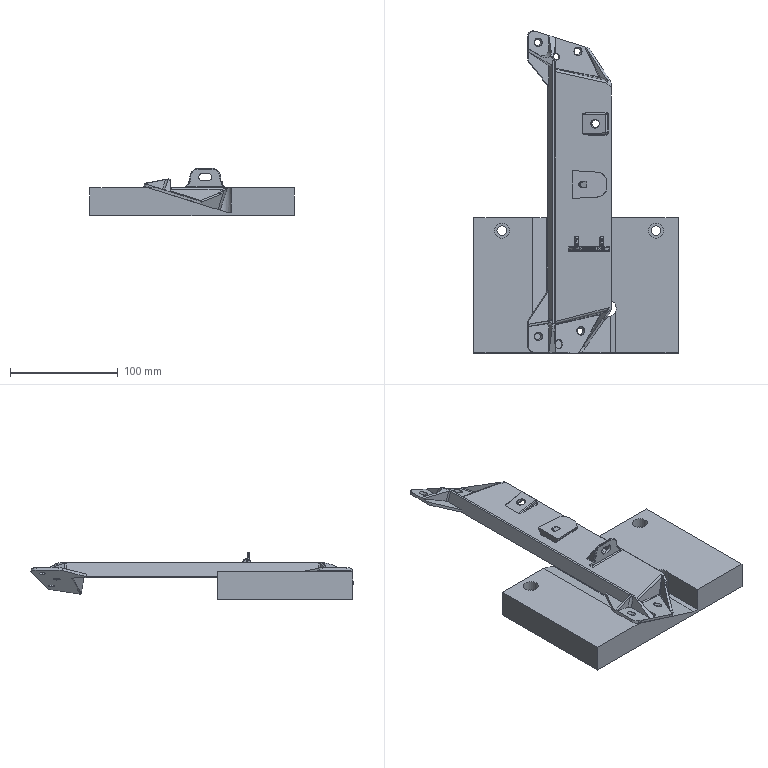NC program | NX | posted with a generic post | part box 190 x 299.709 x 43.804 mm
Whole program:
N10 G17 G21 G94 G90
(L等高精加工_COPY_COPY , TOOL : D6-粗刀)
N12 T01 M6
N14 G53
N16 G17 G0 G90 X-3.185 Y6.75 S6000 M3
N18 G43 Z10. H1
N20 Z0.8
N22 G94 G1 Z-0.2 F2000.
N24 G3 X-3.84 Y8.004 R1.
N26 G1 X-3.901 Y8.023
N28 X-5.822 Y8.626
N30 X-7.135 Y9.039
N32 X-7.149 Y9.042
N34 X-10.361 Y10.05
N36 X-10.489 Y10.096
N38 X-10.596 Y10.128 Z-0.4
N40 X-10.361 Y10.05
N42 X-7.259 Y9.077
N44 X-5.822 Y8.626
N46 X-3.953 Y8.039
N48 X-4.072 Y8.076 Z-0.599
N50 X-5.822 Y8.626
N52 X-7.369 Y9.111
N54 X-10.651 Y10.141
N56 X-10.751 Y10.176
N58 X-10.875 Y10.213 Z-0.699
N60 X-10.998 Y10.251 Z-0.799
N62 X-10.91 Y10.222
N64 X-7.479 Y9.146
N66 X-5.822 Y8.626
N68 X-5.42 Y8.499
N70 X-4.17 Y8.107
N72 X-4.283 Y8.143 Z-0.999
N74 X-5.883 Y8.645
N76 X-7.149 Y9.042
N78 X-7.589 Y9.181
N80 X-7.892 Y9.275
N82 X-10.91 Y10.222
N84 X-11.203 Y10.323
N86 X-11.302 Y10.346 Z-1.099
N88 X-11.399 Y10.378 Z-1.199
N90 X-11.341 Y10.357
N92 X-7.699 Y9.215
N94 X-7.149 Y9.042
N96 X-6.229 Y8.753
N98 X-4.39 Y8.176
N100 X-4.508 Y8.213 Z-1.399
N102 X-6.542 Y8.851
N104 X-7.149 Y9.042
N106 X-7.81 Y9.25
N108 X-11.459 Y10.394
N110 X-11.607 Y10.445
N112 X-11.735 Y10.482 Z-1.499
N114 X-11.862 Y10.522 Z-1.599
N116 X-11.686 Y10.465
N118 X-7.92 Y9.284
N120 X-7.149 Y9.042
N122 X-6.832 Y8.942
N124 X-4.619 Y8.248
N126 X-4.728 Y8.282 Z-1.799
N128 X-7.099 Y9.026
N130 X-7.149 Y9.042
N132 X-8.03 Y9.319
N134 X-12.008 Y10.566
N136 X-12.106 Y10.605
N138 X-12.243 Y10.645 Z-1.899
N140 X-12.378 Y10.694 Z-1.999
N142 X-12.031 Y10.573
N144 X-10.361 Y10.05
N146 X-8.14 Y9.353
N148 X-7.142 Y9.039
N150 X-4.834 Y8.316
N152 X-4.943 Y8.35 Z-2.199
N154 X-8.25 Y9.388
N156 X-12.022 Y10.57
N158 G2 X-12.384 Y10.696 R5.965
N160 G1 X-12.39 Y10.699 Z-2.398
N162 X-12.031 Y10.573
N164 X-8.36 Y9.422
N166 X-5.056 Y8.385
N168 X-5.173 Y8.422 Z-2.598
N170 X-7.142 Y9.039
N172 X-8.47 Y9.457
N174 X-12.031 Y10.573
N176 X-12.376 Y10.693
N178 X-12.396 Y10.701
N180 X-12.402 Y10.704 Z-2.798
N182 X-12.376 Y10.693
N184 X-12.031 Y10.573
N186 X-8.581 Y9.491
N188 X-7.142 Y9.039
N190 X-5.276 Y8.454
N192 X-5.383 Y8.488 Z-2.998
N194 X-7.142 Y9.039
N196 X-8.691 Y9.526
N198 X-12.031 Y10.573
N200 X-12.376 Y10.693
N202 X-12.408 Y10.706
N204 X-12.414 Y10.709 Z-3.198
N206 X-12.376 Y10.693
N208 X-12.031 Y10.573
N210 X-8.801 Y9.56
N212 X-5.492 Y8.522
N214 X-5.6 Y8.556 Z-3.398
N216 X-8.911 Y9.595
N218 X-12.031 Y10.573
N220 X-12.376 Y10.692
N222 X-12.42 Y10.711
N224 X-12.426 Y10.714 Z-3.598
N226 X-12.376 Y10.692
N228 X-12.031 Y10.573
N230 X-9.021 Y9.63
N232 X-5.719 Y8.593
N234 X-5.826 Y8.627 Z-3.798
N236 X-7.142 Y9.039
N238 X-9.131 Y9.664
N240 X-12.031 Y10.573
N242 X-12.376 Y10.692
N244 X-12.432 Y10.716
N246 X-12.438 Y10.719 Z-3.998
N248 X-12.376 Y10.692
N250 X-12.031 Y10.573
N252 X-11.686 Y10.464
N254 X-9.616 Y9.816
N256 X-9.242 Y9.699
N258 X-7.142 Y9.039
N260 X-5.936 Y8.661
N262 X-6.05 Y8.697 Z-4.198
N264 X-7.142 Y9.039
N266 X-9.352 Y9.733
N268 X-12.031 Y10.573
N270 X-12.376 Y10.692
N272 X-12.444 Y10.721
N274 X-12.45 Y10.724 Z-4.398
N276 X-12.376 Y10.692
N278 X-12.031 Y10.573
N280 X-9.462 Y9.768
N282 X-7.142 Y9.039
N284 X-6.16 Y8.731
N286 X-6.262 Y8.763 Z-4.598
N288 X-7.142 Y9.039
N290 X-9.572 Y9.802
N292 X-12.031 Y10.573
N294 X-12.376 Y10.692
N296 X-12.456 Y10.726
N298 X-12.462 Y10.729 Z-4.798
N300 G3 X-12.148 Y10.61 R2.873
N302 G1 X-9.682 Y9.837
N304 X-7.142 Y9.039
N306 X-6.381 Y8.8
N308 X-6.483 Y8.833 Z-4.998
N310 X-9.793 Y9.87
N312 X-12.15 Y10.61
N314 G2 X-12.468 Y10.731 R2.883
N316 G1 X-12.611 Y10.798 Z-5.031
N318 X-12.75 Y10.873 Z-5.063
N320 X-12.887 Y10.956 Z-5.096
N322 X-13.022 Y11.047 Z-5.128
N324 X-13.17 Y11.099 Z-5.161
N326 X-13.324 Y11.127 Z-5.193
N328 X-13.046 Y11.051
N330 X-12.969 Y11.006
N332 G3 X-12.474 Y10.734 R5.001
N334 X-12.151 Y10.61 R2.895
N336 G1 X-9.9 Y9.904
N338 X-6.596 Y8.868
N340 X-6.7 Y8.901 Z-5.376
N342 X-10.001 Y9.936
N344 X-12.151 Y10.611
N346 G2 X-12.48 Y10.736 R2.905
N348 G1 X-12.8 Y10.895
N350 X-12.833 Y10.911
N352 X-13.411 Y11.064
N354 X-13.459 Y11.079
N356 X-13.584 Y11.032 Z-5.558
N358 X-13.411 Y10.979
N360 X-12.501 Y10.738
N362 X-12.031 Y10.573
N364 X-10.102 Y9.967
N366 X-6.798 Y8.931
N368 X-6.901 Y8.964 Z-5.741
N370 X-10.961 Y10.237
N372 G3 X-11.341 Y10.347 R8.846
N374 G1 X-13.468 Y10.911
N376 X-13.712 Y10.978
N378 X-13.838 Y10.927 Z-5.924
N380 X-13.786 Y10.911
N382 X-10.204 Y9.961
N384 X-9.389 Y9.745
N386 X-7.142 Y9.039
N388 X-6.992 Y8.992
N390 X-7.101 Y9.026 Z-6.106
N392 X-7.142 Y9.039
N394 X-7.652 Y9.2
N396 X-10.331 Y9.91
N398 X-13.755 Y10.818
N400 X-13.965 Y10.876
N402 X-14.092 Y10.823 Z-6.289
N404 X-10.457 Y9.86
N406 X-7.405 Y9.05
N408 X-6.983 Y8.939
N410 X-7.073 Y8.878 Z-6.472
N412 X-7.653 Y9.032
N414 X-10.584 Y9.809
N416 X-14.1 Y10.741
N418 X-14.217 Y10.777
N420 X-14.343 Y10.726 Z-6.654
N422 X-14.1 Y10.657
N424 X-10.71 Y9.758
N426 X-7.848 Y9.
N428 X-6.935 Y8.758
N430 G3 X-6.507 Y8.674 R3.326
N432 G1 X-6.387 Y8.628 Z-6.714
N434 X-6.265 Y8.594 Z-6.774
N436 X-6.144 Y8.56 Z-6.834
N438 G2 X-6.857 Y8.655 R3.065
N440 G1 X-8.014 Y8.961
N442 X-10.835 Y9.708
N444 X-14.445 Y10.666
N446 X-14.469 Y10.673
N448 X-14.592 Y10.626 Z-7.013
N450 X-14.445 Y10.583
N452 X-10.958 Y9.659
N454 X-8.159 Y8.917
N456 X-6.857 Y8.572
N458 G3 X-5.874 Y8.475 R2.909
N460 G1 X-5.735 Y8.434 Z-7.101
N462 X-5.595 Y8.389 Z-7.19
N464 G2 X-6.576 Y8.429 R2.801
N466 G1 X-6.857 Y8.49
N468 X-8.287 Y8.869
N470 X-11.081 Y9.61
N472 X-14.715 Y10.574
N474 X-14.829 Y10.529 Z-7.355
N476 X-14.79 Y10.517
N478 X-11.195 Y9.564
N480 X-8.401 Y8.824
N482 X-6.857 Y8.414
N484 X-6.512 Y8.334
N486 G3 X-5.323 Y8.304 R3.003
N488 G1 X-5.196 Y8.265 Z-7.434
N490 X-5.069 Y8.223 Z-7.513
N492 G2 X-6.512 Y8.256 R3.019
N494 G1 X-6.857 Y8.341
N496 X-8.511 Y8.78
N498 X-11.305 Y9.52
N500 X-14.79 Y10.444
N502 X-14.938 Y10.487
N504 X-15.052 Y10.44 Z-7.678
N506 X-14.79 Y10.368
N508 X-11.419 Y9.474
N510 X-8.626 Y8.734
N512 X-6.441 Y8.156
N514 X-6.168 Y8.092
N516 Y8.044 Z-7.77
N518 Y7.999 Z-7.861
N520 X-6.512 Y8.089
N522 X-8.752 Y8.683
N524 X-11.545 Y9.424
N526 X-15.135 Y10.375
N528 X-15.179 Y10.39
N530 X-15.304 Y10.342 Z-8.044
N532 X-15.135 Y10.291
N534 X-11.672 Y9.373
N536 X-8.878 Y8.632
N538 X-6.044 Y7.881
N540 X-5.956 Y7.816 Z-8.135
N542 X-5.867 Y7.751 Z-8.226
N544 X-6.098 Y7.811
N546 X-9.005 Y8.582
N548 X-11.798 Y9.322
N550 X-15.191 Y10.222
N552 X-15.432 Y10.288
N554 X-15.554 Y10.239 Z-8.402
N556 X-15.497 Y10.222
N558 X-11.92 Y9.273
N560 X-5.728 Y7.632
N562 X-5.694 Y7.624
N564 G3 X-4.2 Y7.59 R3.107
N566 G1 X-3.641 Y7.77
N568 X-3.786 Y7.693 Z-8.415
N570 X-3.939 Y7.627 Z-8.428
N572 X-4.098 Y7.569 Z-8.441
N574 X-4.261 Y7.52 Z-8.454
N576 X-4.429 Y7.482 Z-8.467
N578 X-4.598 Y7.456 Z-8.48
N580 X-4.767 Y7.441 Z-8.493
N582 X-4.935 Y7.437 Z-8.506
N584 X-5.099 Y7.451 Z-8.519
N586 X-5.259 Y7.47 Z-8.532
N588 X-5.414 Y7.492 Z-8.545
N590 X-5.564 Y7.517 Z-8.558
N592 X-9.235 Y8.49
N594 X-12.028 Y9.23
N596 X-15.48 Y10.145
N598 X-15.662 Y10.195
N600 X-15.788 Y10.144 Z-8.741
N602 X-15.48 Y10.061
N604 X-12.154 Y9.18
N606 X-9.361 Y8.439
N608 X-5.701 Y7.469
N610 X-5.826 Y7.418 Z-8.924
N612 X-9.487 Y8.388
N614 X-12.281 Y9.129
N616 X-15.825 Y10.068
N618 X-15.914 Y10.096
N620 X-16.04 Y10.046 Z-9.106
N622 X-15.825 Y9.984
N624 X-12.407 Y9.078
N626 X-9.614 Y8.338
N628 X-6.167 Y7.424
N630 X-5.953 Y7.37
N632 X-6.081 Y7.32 Z-9.289
N634 X-6.167 Y7.34
N636 X-12.534 Y9.028
N638 X-16.168 Y9.991
N640 X-16.293 Y9.944 Z-9.472
N642 X-16.17 Y9.907
N644 X-12.66 Y8.977
N646 X-9.867 Y8.236
N648 X-6.209 Y7.268
N650 X-6.336 Y7.22 Z-9.654
N652 X-6.512 Y7.263
N654 X-9.993 Y8.186
N656 X-12.786 Y8.926
N658 X-16.375 Y9.877
N660 X-16.421 Y9.891
N662 X-16.547 Y9.84 Z-9.837
N664 X-16.515 Y9.83
N666 X-12.913 Y8.875
N668 X-10.12 Y8.135
N670 X-6.512 Y7.179
N672 X-6.465 Y7.168
N674 X-6.592 Y7.116 Z-10.02
N676 X-10.246 Y8.084
N678 X-13.039 Y8.825
N680 X-16.515 Y9.746
N682 X-16.673 Y9.792
N684 X-16.8 Y9.74 Z-10.202
N686 X-16.515 Y9.662
N688 X-13.166 Y8.774
N690 X-10.372 Y8.034
N692 X-6.719 Y7.069
N694 X-6.847 Y7.015 Z-10.385
N696 X-10.499 Y7.983
N698 X-13.292 Y8.723
N700 X-16.86 Y9.669
N702 X-16.925 Y9.691
N704 X-17.051 Y9.642 Z-10.568
N706 X-16.86 Y9.585
N708 X-13.419 Y8.673
N710 X-7.202 Y7.025
N712 X-6.973 Y6.969
N714 X-7.101 Y6.918 Z-10.751
N716 X-7.202 Y6.94
N718 X-10.752 Y7.882
N720 X-13.545 Y8.622
N722 X-16.982 Y9.533
N724 X-17.179 Y9.587
N726 X-17.306 Y9.535 Z-10.933
N728 X-13.672 Y8.571
N730 X-10.878 Y7.831
N732 X-7.229 Y6.864
N734 X-7.356 Y6.815 Z-11.116
N736 X-7.547 Y6.863
N738 X-13.798 Y8.521
N740 X-17.205 Y9.424
N742 X-17.432 Y9.486
N744 X-17.559 Y9.434 Z-11.299
N746 X-13.924 Y8.47
N748 X-11.131 Y7.729
N750 X-7.543 Y6.778
N752 X-7.484 Y6.766
N754 X-7.611 Y6.714 Z-11.481
N756 X-11.258 Y7.679
N758 X-14.051 Y8.419
N760 X-17.55 Y9.347
N762 X-17.684 Y9.387
N764 X-17.811 Y9.336 Z-11.664
N766 X-17.55 Y9.263
N768 X-14.177 Y8.369
N770 X-11.384 Y7.628
N772 X-7.892 Y6.702
N774 X-7.738 Y6.665
N776 X-7.865 Y6.613 Z-11.847
N778 X-7.892 Y6.618
N780 X-14.304 Y8.318
N782 X-17.894 Y9.27
N784 X-17.938 Y9.283
N786 X-18.064 Y9.234 Z-12.029
N788 X-17.906 Y9.189
N790 X-14.43 Y8.267
N792 X-11.637 Y7.527
N794 X-8.237 Y6.625
N796 X-7.992 Y6.564
N798 X-8.119 Y6.514 Z-12.212
N800 X-8.237 Y6.541
N802 X-11.763 Y7.476
N804 X-14.557 Y8.217
N806 X-18.191 Y9.18
N808 X-18.317 Y9.132 Z-12.395
N810 X-18.239 Y9.109
N812 X-14.683 Y8.166
N814 X-11.89 Y7.425
N816 X-8.247 Y6.46
N818 X-8.373 Y6.412 Z-12.577
N820 X-8.467 Y6.434
N822 X-12.016 Y7.375
N824 X-14.81 Y8.115
N826 X-18.239 Y9.025
N828 X-18.443 Y9.082
N830 X-18.57 Y9.029 Z-12.76
N832 X-14.936 Y8.065
N834 X-12.143 Y7.324
N836 X-8.582 Y6.38
N838 X-8.5 Y6.362
N840 X-8.627 Y6.311 Z-12.943
N842 X-8.927 Y6.387
N844 X-15.062 Y8.014
N846 X-18.584 Y8.948
N848 X-18.696 Y8.98
N850 X-18.822 Y8.929 Z-13.125
N852 X-18.584 Y8.863
N854 X-15.189 Y7.963
N856 X-8.927 Y6.303
N858 X-8.754 Y6.263
N860 X-8.881 Y6.209 Z-13.308
N862 X-8.927 Y6.219
N864 X-15.315 Y7.913
N866 X-18.929 Y8.871
N868 X-18.949 Y8.877
N870 X-19.076 Y8.826 Z-13.491
N872 X-18.929 Y8.786
N874 X-15.442 Y7.862
N876 X-9.272 Y6.226
N878 X-9.008 Y6.158
N880 X-9.135 Y6.107 Z-13.674
N882 X-9.272 Y6.142
N884 X-15.568 Y7.811
N886 X-18.929 Y8.702
N888 X-19.202 Y8.776
N890 X-19.328 Y8.726 Z-13.856
N892 X-19.274 Y8.709
N894 X-15.695 Y7.761
N896 X-12.901 Y7.02
N898 X-9.262 Y6.056
N900 X-9.388 Y6.008 Z-14.039
N902 X-9.616 Y6.065
N904 X-13.028 Y6.969
N906 X-15.821 Y7.71
N908 X-19.274 Y8.625
N910 X-19.454 Y8.678
N912 X-19.581 Y8.624 Z-14.222
N914 X-19.274 Y8.541
N916 X-15.947 Y7.659
N918 X-13.154 Y6.919
N920 X-9.616 Y5.981
N922 X-9.515 Y5.957
N924 X-9.642 Y5.905 Z-14.404
N926 X-9.961 Y5.988
N928 X-16.074 Y7.608
N930 X-19.619 Y8.548
N932 X-19.707 Y8.575
N934 X-19.834 Y8.523 Z-14.587
N936 X-19.755 Y8.5
N938 X-16.2 Y7.558
N940 X-13.407 Y6.817
N942 X-9.961 Y5.904
N944 X-9.769 Y5.857
N946 X-9.896 Y5.805 Z-14.77
N948 X-9.961 Y5.82
N950 X-13.534 Y6.767
N952 X-16.327 Y7.507
N954 X-19.961 Y8.471
N956 X-20.087 Y8.423 Z-14.952
N958 X-19.964 Y8.387
N960 X-16.453 Y7.456
N962 X-13.66 Y6.716
N964 X-10.023 Y5.752
N966 X-10.149 Y5.705 Z-15.135
N968 X-10.306 Y5.743
N970 X-13.786 Y6.665
N972 X-16.58 Y7.406
N974 X-19.964 Y8.303
N976 X-20.213 Y8.372
N978 X-20.34 Y8.32 Z-15.318
N980 X-20.309 Y8.31
N982 X-16.706 Y7.355
N984 X-13.913 Y6.615
N986 X-10.306 Y5.658
N988 X-10.276 Y5.652
N990 X-10.402 Y5.604 Z-15.5
N992 X-10.651 Y5.666
N994 X-16.833 Y7.304
N996 X-20.309 Y8.226
N998 X-20.466 Y8.271
N1000 X-20.593 Y8.219 Z-15.683
N1002 X-20.361 Y8.156
N1004 X-16.959 Y7.254
N1006 X-10.651 Y5.581
N1008 X-10.528 Y5.554
N1010 X-10.656 Y5.499 Z-15.866
N1012 X-14.292 Y6.462
N1014 X-17.085 Y7.203
N1016 X-20.679 Y8.156
N1018 X-20.719 Y8.168
N1020 X-20.846 Y8.118 Z-16.049
N1022 X-20.654 Y8.065
N1024 X-17.212 Y7.152
N1026 X-10.996 Y5.504
N1028 X-10.782 Y5.45
N1030 X-10.909 Y5.398 Z-16.231
N1032 X-14.545 Y6.361
N1034 X-17.338 Y7.102
N1036 X-20.973 Y8.066
N1038 X-21.098 Y8.018 Z-16.414
N1040 X-20.999 Y7.988
N1042 X-17.465 Y7.051
N1044 X-11.24 Y5.401
N1046 X-11.035 Y5.348
N1048 X-11.162 Y5.299 Z-16.597
N1050 X-11.341 Y5.343
N1052 X-17.591 Y7.
N1054 X-20.999 Y7.904
N1056 X-21.224 Y7.968
N1058 X-21.352 Y7.914 Z-16.779
N1060 X-17.718 Y6.95
N1062 X-11.341 Y5.259
N1064 X-11.288 Y5.248
N1066 X-11.415 Y5.197 Z-16.962
N1068 X-11.686 Y5.266
N1070 X-15.051 Y6.158
N1072 X-17.844 Y6.899
N1074 X-21.344 Y7.827
N1076 X-21.478 Y7.866
N1078 X-21.605 Y7.812 Z-17.145
N1080 X-17.971 Y6.848
N1082 X-15.177 Y6.108
N1084 X-11.686 Y5.182
N1086 X-11.541 Y5.148
N1088 X-11.668 Y5.094 Z-17.327
N1090 X-15.304 Y6.057
N1092 X-18.097 Y6.798
N1094 X-21.689 Y7.75
N1096 X-21.731 Y7.762
N1098 X-21.857 Y7.714 Z-17.51
N1100 X-21.689 Y7.665
N1102 X-18.223 Y6.747
N1104 X-15.43 Y6.006
N1106 X-11.847 Y5.056
N1108 X-11.795 Y5.044
N1110 X-11.921 Y4.996 Z-17.693
N1112 X-12.031 Y5.021
N1114 X-15.557 Y5.956
N1116 X-18.35 Y6.696
N1118 X-21.689 Y7.581
N1120 X-21.984 Y7.661
N1122 X-22.11 Y7.612 Z-17.875
N1124 X-22.033 Y7.589
N1126 X-18.476 Y6.646
N1128 X-12.376 Y5.028
N1130 X-12.048 Y4.942
N1132 X-12.173 Y4.896 Z-18.058
N1134 X-12.376 Y4.944
N1136 X-15.81 Y5.854
N1138 X-18.603 Y6.595
N1140 X-22.033 Y7.504
N1142 X-22.236 Y7.561
N1144 X-22.363 Y7.508 Z-18.241
N1146 X-18.729 Y6.544
N1148 X-15.936 Y5.804
N1150 X-12.376 Y4.86
N1152 X-12.3 Y4.844
N1154 X-12.427 Y4.79 Z-18.423
N1156 X-12.721 Y4.867
N1158 X-18.856 Y6.494
N1160 X-22.378 Y7.427
N1162 X-22.49 Y7.458
N1164 X-22.616 Y7.408 Z-18.606
N1166 X-22.378 Y7.343
N1168 X-18.982 Y6.443
N1170 X-16.189 Y5.702
N1172 X-12.554 Y4.74
N1174 X-12.68 Y4.69 Z-18.789
N1176 X-12.721 Y4.699
N1178 X-16.315 Y5.652
N1180 X-19.109 Y6.392
N1182 X-22.723 Y7.35
N1184 X-22.742 Y7.357
N1186 X-22.868 Y7.31 Z-18.972
N1188 X-22.723 Y7.266
N1190 X-19.235 Y6.341
N1192 X-13.066 Y4.706
N1194 X-12.806 Y4.64
N1196 X-12.933 Y4.59 Z-19.154
N1198 X-13.066 Y4.622
N1200 X-16.568 Y5.55
N1202 X-19.361 Y6.291
N1204 X-22.723 Y7.182
N1206 X-22.995 Y7.257
N1208 X-23.122 Y7.206 Z-19.337
N1210 X-23.068 Y7.189
N1212 X-19.488 Y6.24
N1214 X-16.695 Y5.5
N1216 X-13.06 Y4.536
N1218 X-13.186 Y4.489 Z-19.52
N1220 X-13.411 Y4.545
N1222 X-16.821 Y5.449
N1224 X-19.614 Y6.189
N1226 X-23.134 Y7.123
N1228 X-23.248 Y7.156
N1230 X-23.375 Y7.103 Z-19.702
N1232 X-19.741 Y6.139
N1234 X-13.411 Y4.461
N1236 X-13.312 Y4.438
N1238 X-13.439 Y4.384 Z-19.885
N1240 X-17.074 Y5.348
N1242 X-19.867 Y6.088
N1244 X-23.413 Y7.028
N1246 X-23.501 Y7.054
N1248 X-23.627 Y7.004 Z-20.068
N1250 X-23.413 Y6.944
N1252 X-19.994 Y6.037
N1254 X-17.2 Y5.297
N1256 X-13.695 Y4.368
N1258 X-13.565 Y4.337
N1260 X-13.692 Y4.285 Z-20.25
N1262 X-17.327 Y5.246
N1264 X-20.12 Y5.987
N1266 X-23.754 Y6.95
N1268 X-23.88 Y6.902 Z-20.433
N1270 X-23.758 Y6.867
N1272 X-20.247 Y5.936
N1274 X-17.453 Y5.195
N1276 X-13.818 Y4.235
N1278 X-13.944 Y4.187 Z-20.616
N1280 X-14.1 Y4.222
N1282 X-20.373 Y5.885
N1284 X-23.758 Y6.783
N1286 X-24.007 Y6.851
N1288 X-24.133 Y6.8 Z-20.798
N1290 X-24.103 Y6.79
N1292 X-20.499 Y5.835
N1294 X-14.1 Y4.138
N1296 X-14.071 Y4.132
N1298 X-14.198 Y4.082 Z-20.981
N1300 X-14.445 Y4.145
N1302 X-20.626 Y5.784
N1304 X-24.103 Y6.706
N1306 X-24.26 Y6.749
N1308 X-24.386 Y6.698 Z-21.164
N1310 X-24.103 Y6.622
N1312 X-20.752 Y5.733
N1314 X-17.959 Y4.993
N1316 X-14.324 Y4.03
N1318 X-14.451 Y3.979 Z-21.347
N1320 X-18.086 Y4.942
N1322 X-20.879 Y5.683
N1324 X-24.448 Y6.629
N1326 X-24.512 Y6.649
N1328 X-24.638 Y6.6 Z-21.529
N1330 X-24.448 Y6.545
N1332 X-21.005 Y5.632
N1334 X-18.212 Y4.891
N1336 X-14.79 Y3.984
N1338 X-14.577 Y3.931
N1340 X-14.703 Y3.88 Z-21.712
N1342 X-14.79 Y3.9
N1344 X-21.132 Y5.581
N1346 X-24.448 Y6.46
N1348 X-24.765 Y6.546
N1350 X-24.891 Y6.497 Z-21.895
N1352 X-24.793 Y6.468
N1354 X-21.258 Y5.531
N1356 X-15.135 Y3.907
N1358 X-14.83 Y3.828
N1360 X-14.956 Y3.78 Z-22.077
N1362 X-15.135 Y3.823
N1364 X-18.591 Y4.739
N1366 X-21.385 Y5.48
N1368 X-24.983 Y6.434
N1370 X-25.018 Y6.444
N1372 X-25.145 Y6.393 Z-22.26
N1374 X-21.511 Y5.429
N1376 X-18.718 Y4.689
N1378 X-15.135 Y3.739
N1380 X-15.083 Y3.727
N1382 X-15.209 Y3.675 Z-22.443
N1384 X-18.844 Y4.638
N1386 X-21.637 Y5.379
N1388 X-25.138 Y6.306
N1390 X-25.27 Y6.345
N1392 X-25.397 Y6.294 Z-22.625
N1394 X-25.138 Y6.222
N1396 X-21.764 Y5.328
N1398 X-18.971 Y4.587
N1400 X-15.335 Y3.628
N1402 X-15.463 Y3.574 Z-22.808
N1404 X-19.097 Y4.537
N1406 X-21.89 Y5.277
N1408 X-25.483 Y6.23
N1410 X-25.524 Y6.243
N1412 X-25.65 Y6.193 Z-22.991
N1414 X-25.483 Y6.145
N1416 X-22.017 Y5.227
N1418 X-19.223 Y4.486
N1420 X-15.825 Y3.585
N1422 X-15.588 Y3.527
N1424 X-15.715 Y3.477 Z-23.173
N1426 X-15.825 Y3.501
N1428 X-22.143 Y5.176
N1430 X-25.589 Y6.089
N1432 X-25.777 Y6.141
N1434 X-25.904 Y6.089 Z-23.356
N1436 X-22.27 Y5.125
N1438 X-19.476 Y4.385
N1440 X-15.842 Y3.421
N1442 X-15.968 Y3.372 Z-23.539
N1444 X-16.17 Y3.424
N1446 X-19.603 Y4.334
N1448 X-22.396 Y5.074
N1450 X-25.828 Y5.984
N1452 X-26.029 Y6.04
N1454 X-26.156 Y5.987 Z-23.722
N1456 X-22.523 Y5.024
N1458 X-16.151 Y3.334
N1460 X-16.094 Y3.322
N1462 X-16.221 Y3.271 Z-23.904
N1464 X-16.468 Y3.334
N1466 X-19.856 Y4.233
N1468 X-22.649 Y4.973
N1470 X-26.172 Y5.907
N1472 X-26.281 Y5.941
N1474 X-26.408 Y5.89 Z-24.087
N1476 X-26.172 Y5.823
N1478 X-22.775 Y4.922
N1480 X-16.515 Y3.263
N1482 X-16.347 Y3.222
N1484 X-16.473 Y3.17 Z-24.27
N1486 X-16.515 Y3.178
N1488 X-22.902 Y4.872
N1490 X-26.517 Y5.83
N1492 X-26.535 Y5.836
N1494 X-26.661 Y5.788 Z-24.452
N1496 X-26.517 Y5.746
N1498 X-23.028 Y4.821
N1500 X-20.235 Y4.081
N1502 X-16.86 Y3.186
N1504 X-16.6 Y3.12
N1506 X-16.726 Y3.07 Z-24.635
N1508 X-16.86 Y3.101
N1510 X-20.361 Y4.03
N1512 X-23.155 Y4.77
N1514 X-26.788 Y5.734
N1516 X-26.914 Y5.684 Z-24.818
N1518 X-26.862 Y5.669
N1520 X-23.281 Y4.72
N1522 X-20.488 Y3.979
N1524 X-16.853 Y3.016
N1526 X-16.979 Y2.967 Z-25.
N1528 X-17.075 Y2.99
N1530 X-20.614 Y3.928
N1532 X-23.408 Y4.669
N1534 X-26.862 Y5.585
N1536 X-27.04 Y5.636
N1538 X-27.167 Y5.583 Z-25.183
N1540 X-26.862 Y5.501
N1542 X-23.534 Y4.618
N1544 X-20.741 Y3.878
N1546 X-17.205 Y2.94
N1548 X-17.105 Y2.918
N1550 X-17.232 Y2.865 Z-25.366
N1552 X-17.55 Y2.948
N1554 X-23.661 Y4.568
N1556 X-27.207 Y5.508
N1558 X-27.292 Y5.534
N1560 X-27.419 Y5.483 Z-25.548
N1562 X-27.207 Y5.424
N1564 X-23.787 Y4.517
N1566 X-17.55 Y2.863
N1568 X-17.358 Y2.818
N1570 X-17.484 Y2.765 Z-25.731
N1572 X-21.12 Y3.726
N1574 X-23.913 Y4.466
N1576 X-27.546 Y5.43
N1578 X-27.672 Y5.38 Z-25.914
N1580 X-27.552 Y5.347
N1582 X-24.04 Y4.416
N1584 X-21.247 Y3.675
N1586 X-17.894 Y2.786
N1588 X-17.611 Y2.713
N1590 X-17.738 Y2.662 Z-26.096
N1592 X-17.894 Y2.702
N1594 X-24.166 Y4.365
N1596 X-27.552 Y5.263
N1598 X-27.798 Y5.33
N1600 X-27.924 Y5.278 Z-26.279
N1602 X-27.897 Y5.27
N1604 X-24.293 Y4.314
N1606 X-17.894 Y2.618
N1608 X-17.864 Y2.612
N1610 X-17.99 Y2.562 Z-26.462
N1612 X-18.239 Y2.625
N1614 X-21.626 Y3.523
N1616 X-24.419 Y4.264
N1618 X-27.897 Y5.186
N1620 X-28.049 Y5.231
N1622 X-28.176 Y5.179 Z-26.645
N1624 X-27.897 Y5.101
N1626 X-24.546 Y4.213
N1628 X-18.239 Y2.541
N1630 X-18.116 Y2.512
N1632 X-18.243 Y2.458 Z-26.827
N1634 X-21.879 Y3.422
N1636 X-24.672 Y4.162
N1638 X-28.242 Y5.108
N1640 X-28.303 Y5.127
N1642 X-28.429 Y5.076 Z-27.01
N1644 X-28.363 Y5.056
N1646 X-24.798 Y4.112
N1648 X-22.005 Y3.371
N1650 X-18.584 Y2.464
N1652 X-18.369 Y2.411
N1654 X-18.496 Y2.359 Z-27.193
N1656 X-18.584 Y2.38
N1658 X-22.132 Y3.32
N1660 X-24.925 Y4.061
N1662 X-28.556 Y5.024
N1664 X-28.678 Y4.974 Z-27.375
N1666 X-28.587 Y4.947
N1668 X-25.051 Y4.01
N1670 X-22.258 Y3.27
N1672 X-18.623 Y2.306
N1674 X-18.748 Y2.259 Z-27.558
N1676 X-18.923 Y2.301
N1678 X-25.178 Y3.96
N1680 X-28.587 Y4.863
N1682 X-28.799 Y4.922
N1684 X-28.921 Y4.867 Z-27.741
N1686 X-28.587 Y4.778
N1688 X-25.304 Y3.909
N1690 X-18.929 Y2.219
N1692 X-18.875 Y2.207
N1694 X-19. Y2.157 Z-27.923
N1696 X-19.274 Y2.226
N1698 X-25.43 Y3.858
N1700 X-28.932 Y4.784
N1702 X-29.04 Y4.816
N1704 X-29.159 Y4.762 Z-28.104
N1706 X-25.556 Y3.808
N1708 X-22.763 Y3.067
N1710 X-19.274 Y2.143
N1712 X-19.125 Y2.109
N1714 X-19.252 Y2.054 Z-28.286
N1716 X-19.274 Y2.059
N1718 X-22.888 Y3.017
N1720 X-25.682 Y3.758
N1722 X-28.587 Y4.526
N1724 X-29.287 Y4.709
N1726 X-29.353 Y4.643 Z-28.467
N1728 X-25.807 Y3.707
N1730 X-23.014 Y2.967
N1732 X-19.619 Y2.067
N1734 X-19.377 Y2.004
N1736 X-19.502 Y1.953 Z-28.648
N1738 X-23.139 Y2.917
N1740 X-25.932 Y3.657
N1742 X-29.52 Y4.603
N1744 X-29.628 Y4.547 Z-28.829
N1746 X-26.057 Y3.607
N1748 X-23.264 Y2.866
N1750 X-19.627 Y1.903
N1752 X-19.749 Y1.856 Z-29.006
N1754 X-19.964 Y1.91
N1756 X-23.387 Y2.817
N1758 X-26.18 Y3.558
N1760 X-29.277 Y4.373
N1762 X-29.638 Y4.462
N1764 X-29.568 Y4.397 Z-29.095
N1766 X-29.498 Y4.322 Z-29.183
N1768 G2 X-29.296 Y4.292 R1.067
N1770 G1 X-28.932 Y4.202
N1772 X-26.302 Y3.509
N1774 X-23.509 Y2.768
N1776 X-19.871 Y1.807
N1778 X-19.986 Y1.759 Z-29.349
N1780 X-20.309 Y1.843
N1782 X-23.624 Y2.722
N1784 X-26.417 Y3.463
N1786 X-28.587 Y4.035
N1788 X-28.932 Y4.124
N1790 X-29.277 Y4.182
N1792 X-29.343 Y4.186
N1794 X-29.217 Y4.112 Z-29.431
N1796 X-29.092 Y4.035 Z-29.514
N1798 G2 X-28.587 Y3.959 R1.885
N1800 G1 X-26.531 Y3.417
N1802 X-23.738 Y2.676
N1804 X-20.309 Y1.767
N1806 X-20.1 Y1.715
N1808 X-20.21 Y1.67 Z-29.674
N1810 X-20.309 Y1.693
N1812 X-23.849 Y2.632
N1814 X-26.642 Y3.372
N1816 X-28.242 Y3.794
N1818 X-28.511 Y3.859
N1820 G3 X-28.815 Y3.877 R0.861
N1822 G1 X-28.668 Y3.782 Z-29.758
N1824 X-28.522 Y3.693 Z-29.842
N1826 X-28.433 Y3.737
N1828 X-28.114 Y3.679
N1830 X-26.759 Y3.326
N1832 X-23.965 Y2.585
N1834 X-20.327 Y1.621
N1836 X-20.402 Y1.592 Z-29.951
N1838 X-20.486 Y1.613
N1840 X-24.041 Y2.555
N1842 X-27.508 Y3.474
N1844 G3 X-28.25 Y3.639 R9.165
N1846 G1 X-28.677 Y3.425
N1848 X-28.751 Y3.288 Z-30.005
N1850 X-28.828 Y3.157 Z-30.059
N1852 X-28.072 Y3.542
N1854 G2 X-27.737 Y3.479 R2.515
N1856 G1 X-26.909 Y3.266
N1858 X-24.115 Y2.525
N1860 X-20.654 Y1.607
N1862 X-20.476 Y1.565
N1864 X-20.55 Y1.534 Z-30.167
N1866 X-20.654 Y1.558
N1868 X-24.19 Y2.495
N1870 X-26.983 Y3.236
N1872 X-27.725 Y3.42
N1874 X-27.897 Y3.445
N1876 X-28.932 Y2.91
N1878 X-28.979 Y2.888
N1880 X-29.056 Y2.751 Z-30.221
N1882 X-29.134 Y2.618 Z-30.275
N1884 X-27.725 Y3.345
N1886 G2 X-27.293 Y3.268 R2.668
N1888 G1 X-24.265 Y2.465
N1890 X-20.654 Y1.508
N1892 X-20.625 Y1.502
N1894 X-20.699 Y1.473 Z-30.383
N1896 X-20.999 Y1.55
N1898 X-24.339 Y2.435
N1900 X-27.133 Y3.176
N1902 X-27.207 Y3.191
N1904 X-27.535 Y3.251
N1906 X-29.277 Y2.354
N1908 X-29.453 Y2.276
N1910 X-29.568 Y2.188 Z-30.404
N1912 X-29.689 Y2.111 Z-30.426
N1914 X-29.81 Y2.036 Z-30.447
N1916 X-29.934 Y1.966 Z-30.469
N1918 X-30.06 Y1.91 Z-30.49
N1920 G3 X-29.011 Y2.301 R4.743
N1922 G1 X-27.552 Y3.056
N1924 X-27.356 Y3.154
N1926 X-26.962 Y3.081
N1928 X-24.414 Y2.406
N1930 X-20.999 Y1.5
N1932 X-20.773 Y1.445
N1934 X-20.848 Y1.416 Z-30.598
N1936 X-20.999 Y1.45
N1938 X-24.489 Y2.376
N1940 X-26.783 Y2.984
N1942 G3 X-27.176 Y3.058 R2.61
N1944 G1 X-27.207 Y3.045
N1946 X-28.643 Y2.301
N1948 X-28.932 Y2.157
N1950 G2 X-30.513 Y1.689 R5.033
N1952 G1 X-30.633 Y1.627 Z-30.634
N1954 X-30.754 Y1.579 Z-30.67
N1956 X-30.876 Y1.543 Z-30.706
N1958 G3 X-28.587 Y2.142 R5.269
N1960 G1 X-27.002 Y2.961
N1962 G2 X-26.605 Y2.887 R2.628
N1964 G1 X-24.563 Y2.346
N1966 X-20.999 Y1.401
N1968 X-20.923 Y1.384
N1970 X-20.998 Y1.351 Z-30.814
N1972 X-24.638 Y2.316
N1974 X-26.426 Y2.79
N1976 X-26.823 Y2.864
N1978 X-28.418 Y2.042
N1980 G2 X-31.178 Y1.444 R5.425
N1982 G1 X-31.311 Y1.399 Z-30.868
N1984 X-31.443 Y1.373 Z-30.922
N1986 G3 X-28.4 Y1.867 R5.612
N1988 G1 X-28.242 Y1.941
N1990 X-26.645 Y2.767
N1992 X-26.283 Y2.701
N1994 X-26.248 Y2.693
N1996 X-24.713 Y2.286
N1998 X-21.344 Y1.393
N2000 X-21.072 Y1.322
N2002 X-21.146 Y1.292 Z-31.03
N2004 X-21.344 Y1.343
N2006 X-24.787 Y2.256
N2008 X-26.069 Y2.596
N2010 G3 X-26.468 Y2.67 R3.793
N2012 G1 X-28.242 Y1.758
N2014 X-28.568 Y1.613
N2016 G2 X-31.681 Y1.321 R6.236
N2018 G1 X-31.784 Y1.301 Z-31.084
N2020 X-31.886 Y1.291 Z-31.138
N2022 G3 X-30.12 Y1.157 R7.407
N2024 X-27.861 Y1.76 R5.436
N2026 G1 X-26.291 Y2.572
N2028 G2 X-25.891 Y2.499 R3.983
N2030 G1 X-24.862 Y2.226
N2032 X-21.25 Y1.268
N2034 X-21.221 Y1.262
N2036 X-21.295 Y1.233 Z-31.246
N2038 X-21.344 Y1.243
N2040 X-24.937 Y2.196
N2042 X-25.712 Y2.402
N2044 X-26.114 Y2.475
N2046 X-27.78 Y1.613
N2048 G2 X-29.967 Y1.059 R5.326
N2050 X-32.078 Y1.267 R8.052
N2052 G1 X-32.191 Y1.244 Z-31.353
N2054 G3 X-30.311 Y0.957 R8.741
N2056 X-27.552 Y1.542 R5.503
N2058 G1 X-27.412 Y1.613
N2060 X-25.936 Y2.378
N2062 X-25.534 Y2.305
N2064 X-25.011 Y2.166
N2066 X-21.625 Y1.268
N2068 X-21.37 Y1.202
N2070 X-21.444 Y1.173 Z-31.461
N2072 X-21.689 Y1.236
N2074 X-25.086 Y2.136
N2076 X-25.355 Y2.208
N2078 X-25.752 Y2.281
N2080 X-25.766 Y2.277
N2082 X-26.023 Y2.143
N2084 X-27.552 Y1.357
N2086 X-27.747 Y1.268
N2088 G2 X-30.656 Y0.896 R5.893
N2090 X-32.304 Y1.22 R11.403
N2092 G1 X-32.403 Y1.195 Z-31.569
N2094 G3 X-31.001 Y0.872 R17.172
N2096 X-27.897 Y1.048 R6.398
N2098 G1 X-27.552 Y1.18
N2100 X-26.172 Y1.876
N2102 X-25.587 Y2.18
N2104 X-25.573 Y2.184
N2106 X-25.138 Y2.1
N2108 X-21.689 Y1.186
N2110 X-21.518 Y1.144
N2112 X-21.592 Y1.114 Z-31.677
N2114 X-21.689 Y1.136
N2116 X-25.035 Y2.023
N2118 G3 X-25.407 Y2.083 R1.909
N2120 G1 X-26.947 Y1.284
N2122 G2 X-27.897 Y0.891 R5.887
N2124 X-31.001 Y0.807 R6.639
N2126 X-32.471 Y1.166 R20.631
N2128 G1 X-32.541 Y1.136 Z-31.785
N2130 X-32.381 Y1.089
N2132 X-31.346 Y0.823
N2134 G3 X-29.528 Y0.564 R8.72
N2136 X-26.773 Y1.184 R5.542
N2138 G1 X-25.228 Y1.987
N2140 G2 X-24.935 Y1.943 R1.405
N2142 G1 X-24.448 Y1.818
N2144 X-21.689 Y1.087
N2146 X-21.667 Y1.082
N2148 X-21.741 Y1.053 Z-31.893
N2150 X-22.033 Y1.129
N2152 X-24.103 Y1.676
N2154 X-24.763 Y1.847
N2156 G3 X-25.05 Y1.889 R1.341
N2158 G1 X-26.62 Y1.074
N2160 G2 X-28.86 Y0.477 R5.342
N2162 X-31.001 Y0.688 R7.717
N2164 X-32.61 Y1.104 R38.331
N2166 G1 X-32.68 Y1.071 Z-32.001
N2168 G3 X-30.786 Y0.58 R62.763
N2170 X-28.587 Y0.386 R7.73
N2172 X-26.514 Y0.939 R5.264
N2174 G1 X-24.871 Y1.793
N2176 X-24.793 Y1.786
N2178 X-24.103 Y1.627
N2180 X-22.033 Y1.079
N2182 X-21.815 Y1.024
N2184 X-21.889 Y0.994 Z-32.109
N2186 X-24.151 Y1.589
N2188 G3 X-24.693 Y1.695 R4.445
N2190 G1 X-26.335 Y0.842
N2192 G2 X-28.587 Y0.277 R5.431
N2194 X-30.656 Y0.497 R7.794
N2196 G1 X-31.001 Y0.577
N2198 X-32.726 Y1.031
N2200 X-32.75 Y1.039
N2202 X-32.819 Y1.009 Z-32.216
N2204 X-32.726 Y0.982
N2206 X-30.656 Y0.441
N2208 X-30.282 Y0.356
N2210 G3 X-28.455 Y0.181 R7.174
N2212 G1 X-28.242 Y0.188
N2214 G3 X-26.157 Y0.745 R5.347
N2216 G1 X-24.514 Y1.598
N2218 X-24.501 Y1.602
N2220 X-24.103 Y1.524
N2222 X-21.963 Y0.963
N2224 X-22.038 Y0.931 Z-32.324
N2226 G3 X-24.103 Y1.466 R71.614
N2228 G1 X-24.323 Y1.505
N2230 X-24.337 Y1.501
N2232 X-25.978 Y0.648
N2234 G2 X-27.897 Y0.108 R5.204
N2236 X-30.311 Y0.305 R7.366
N2238 G1 X-30.656 Y0.387
N2240 X-32.726 Y0.932
N2242 X-32.888 Y0.979
N2244 X-32.958 Y0.945 Z-32.432
N2246 X-32.884 Y0.924
N2248 X-30.656 Y0.336
N2250 X-30.261 Y0.235
N2252 G3 X-27.897 Y-0.002 R7.759
N2254 X-25.8 Y0.551 R5.308
N2256 G1 X-24.159 Y1.403
N2258 X-24.145 Y1.407
N2260 X-23.758 Y1.328
N2262 X-23.503 Y1.268
N2264 X-22.198 Y0.924
N2266 X-22.112 Y0.903
N2268 X-22.186 Y0.875 Z-32.54
N2270 X-22.378 Y0.922
N2272 X-23.542 Y1.229
N2274 G3 X-23.98 Y1.306 R2.68
N2276 G1 X-25.621 Y0.454
N2278 G2 X-28.441 Y-0.11 R5.67
N2280 X-30.195 Y0.166 R9.176
N2282 G1 X-30.656 Y0.285
N2284 X-33.028 Y0.912
N2286 X-33.097 Y0.882 Z-32.648
N2288 X-30.311 Y0.146
N2290 X-29.967 Y0.056
N2292 G3 X-27.552 Y-0.196 R7.855
N2294 X-25.443 Y0.357 R5.336
N2296 G1 X-24.049 Y1.081
N2298 X-23.788 Y1.213
N2300 X-23.241 Y1.099
N2302 X-22.378 Y0.872
N2304 X-22.26 Y0.845
N2306 X-22.335 Y0.813 Z-32.756
N2308 X-23.241 Y1.046
N2310 X-23.609 Y1.116
N2312 X-23.654 Y1.096
N2314 X-24.198 Y0.814
N2316 X-25.264 Y0.26
N2318 G2 X-27.207 Y-0.277 R5.154
N2320 G1 X-27.37 Y-0.287
N2322 G2 X-29.628 Y-0.079 R7.523
N2324 G1 X-29.967 Y0.005
N2326 X-33.071 Y0.824
N2328 X-33.166 Y0.852
N2330 X-33.235 Y0.822 Z-32.864
N2332 X-33.071 Y0.774
N2334 X-29.967 Y-0.046
N2336 X-29.622 Y-0.135
N2338 G3 X-27.207 Y-0.388 R7.743
N2340 X-25.086 Y0.163 R5.295
N2342 G1 X-24.347 Y0.547
N2344 X-23.43 Y1.019
N2346 X-23.241 Y0.988
N2348 X-22.409 Y0.782
N2350 X-22.483 Y0.751 Z-32.972
N2352 G3 X-23.258 Y0.921 R7.054
N2354 G1 X-24.496 Y0.279
N2356 X-24.907 Y0.066
N2358 G2 X-27.369 Y-0.499 R5.619
N2360 X-29.277 Y-0.273 R8.214
N2362 G1 X-29.967 Y-0.097
N2364 X-33.071 Y0.725
N2366 X-33.305 Y0.79
N2368 X-33.374 Y0.757 Z-33.08
N2370 X-33.071 Y0.675
N2372 X-29.967 Y-0.147
N2374 X-29.277 Y-0.325
N2376 G3 X-26.819 Y-0.58 R7.949
N2378 X-24.651 Y0.01 R5.326
N2380 G1 X-23.219 Y0.752
N2382 X-23.068 Y0.824
N2384 G2 X-22.488 Y0.701 R4.729
N2386 G1 X-22.491 Y0.677 Z-33.133
N2388 X-22.494 Y0.648 Z-33.187
N2390 X-22.891 Y0.728
N2392 X-24.448 Y-0.075
N2394 G2 X-26.862 Y-0.685 R5.357
N2396 X-28.974 Y-0.454 R8.058
N2398 G1 X-29.277 Y-0.377
N2400 X-33.416 Y0.717
N2402 X-33.444 Y0.726
N2404 X-33.513 Y0.696 Z-33.295
N2406 X-33.416 Y0.667
N2408 X-29.277 Y-0.429
N2410 X-29.186 Y-0.454
N2412 G3 X-26.857 Y-0.789 R8.987
N2414 X-24.29 Y-0.181 R5.451
N2416 G1 X-22.723 Y0.629
N2418 X-22.713 Y0.631
N2420 X-22.499 Y0.595
N2422 X-22.448 Y0.52 Z-33.403
N2424 X-22.534 Y0.534
N2426 X-22.551 Y0.528
N2428 X-24.086 Y-0.264
N2430 G2 X-26.329 Y-0.87 R5.505
N2432 X-28.587 Y-0.653 R7.723
N2434 G1 X-29.277 Y-0.479
N2436 X-33.416 Y0.617
N2438 X-33.582 Y0.665
N2440 X-33.652 Y0.633 Z-33.511
N2442 X-33.462 Y0.58
N2444 X-29.277 Y-0.529
N2446 X-28.587 Y-0.706
N2448 G3 X-27.207 Y-0.944 R7.91
N2450 G1 X-26.862 Y-0.977
N2452 G3 X-24.448 Y-0.608 R6.017
N2454 G1 X-24.103 Y-0.461
N2456 X-22.378 Y0.428
N2458 X-22.359 Y0.436
N2460 X-22.264 Y0.392 Z-33.565
N2462 X-22.168 Y0.345 Z-33.619
N2464 X-23.758 Y-0.472
N2466 G2 X-26.517 Y-1.075 R5.533
N2468 X-28.587 Y-0.759 R9.001
N2470 G1 X-33.679 Y0.588
N2472 Y0.538 Z-33.727
N2474 X-28.587 Y-0.811
N2476 G3 X-27.207 Y-1.102 R13.483
N2478 X-24.103 Y-0.811 R6.218
N2480 G1 X-23.758 Y-0.656
N2482 X-22.02 Y0.235
N2484 X-21.94 Y0.251
N2486 X-21.85 Y0.225 Z-33.778
N2488 X-21.755 Y0.179 Z-33.829
N2490 X-21.861 Y0.139
N2492 X-23.413 Y-0.663
N2494 G2 X-25.483 Y-1.244 R5.224
N2496 X-27.897 Y-1.032 R7.667
N2498 G1 X-28.587 Y-0.858
N2500 X-33.679 Y0.491
N2502 Y0.445 Z-33.931
N2504 X-27.897 Y-1.083
N2506 G3 X-25.138 Y-1.317 R7.701
N2508 X-23.329 Y-0.798 R5.119
N2510 G1 X-21.661 Y0.063
N2512 X-21.583 Y0.1
N2514 X-21.426 Y0.095 Z-33.982
N2516 X-21.267 Y0.086 Z-34.032
N2518 X-23.068 Y-0.841
N2520 X-23.184 Y-0.897
N2522 G2 X-25.871 Y-1.448 R5.687
N2524 X-27.868 Y-1.142 R9.11
N2526 G1 X-33.679 Y0.398
N2528 Y0.35 Z-34.134
N2530 X-27.897 Y-1.182
N2532 X-27.552 Y-1.269
N2534 G3 X-25.671 Y-1.542 R8.636
N2536 X-23.068 Y-1.016 R5.739
N2538 G1 X-21.689 Y-0.309
N2540 X-21.358 Y-0.137
N2542 G2 X-20.01 Y-0.564 R1.
N2544 G1 Z-33.134
N2546 G0 Z10.
N2548 M5
N2550 M2